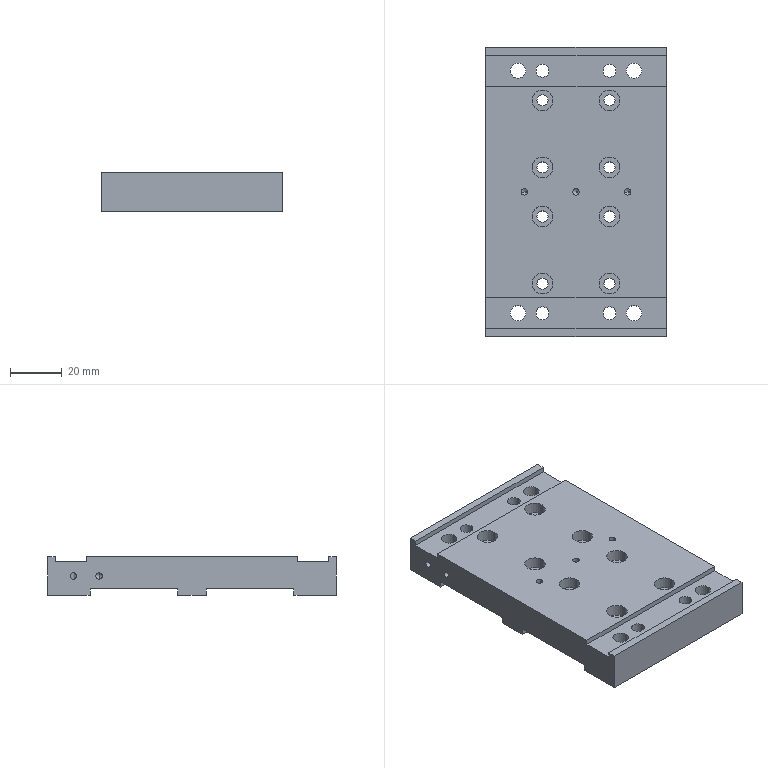Part | SolidWorks | features HoleWzd 8, ICE 4, MirrorPattern 2, Extrusion 1 | 1 solid | 98 faces | box 70 x 112 x 15 mm | volume 96794 mm3 | cylinder 59 | plane 30 | cone 9 | commonest cylinder face diameters 4.3 x16 8 x16 2.5 x11 5 x8 6 x8